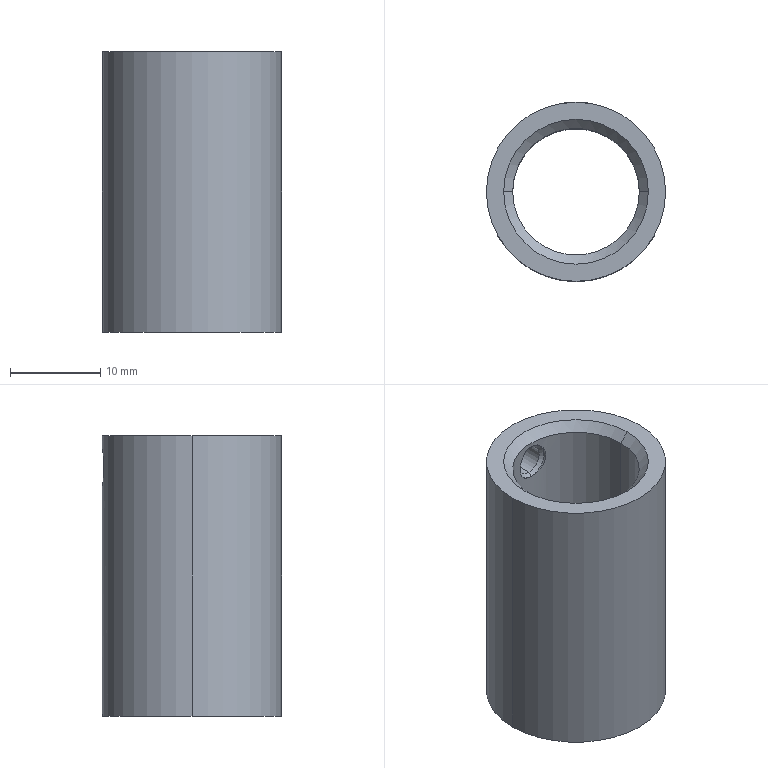Part | SolidWorks | features RefAxis 9, 3DProfileFeature 3, RevCut 1, Revolution 1 | 1 solid | 16 faces | box 19.8 x 19.8 x 31 mm | volume 4724 mm3 | cylinder 8 | cone 6 | plane 2 | commonest cylinder face diameters 3.242 x2 4 x2 14 x2 19.8 x2
STEP:
#1=CARTESIAN_POINT('',(0.,7.379,13.879));
#2=VERTEX_POINT('',#1);
#3=CARTESIAN_POINT('',(0.,7.379,17.121));
#4=VERTEX_POINT('',#3);
#5=CARTESIAN_POINT('',(0.,7.379,15.5));
#6=DIRECTION('',(0.,1.,0.));
#7=DIRECTION('',(0.,0.,1.));
#8=AXIS2_PLACEMENT_3D('',#5,#6,#7);
#9=CIRCLE('',#8,1.621);
#10=EDGE_CURVE('',#2,#4,#9,.T.);
#11=ORIENTED_EDGE('',*,*,#10,.T.);
#12=CARTESIAN_POINT('',(0.,7.,17.5));
#13=VERTEX_POINT('',#12);
#14=CARTESIAN_POINT('',(0.,7.,17.5));
#15=DIRECTION('',(0.,-0.7071,0.7071));
#16=VECTOR('',#15,1000.);
#17=LINE('',#14,#16);
#18=EDGE_CURVE('',#4,#13,#17,.T.);
#19=ORIENTED_EDGE('',*,*,#18,.T.);
#20=CARTESIAN_POINT('',(0.,7.,13.5));
#21=VERTEX_POINT('',#20);
#22=CARTESIAN_POINT('',(0.,7.,15.5));
#23=DIRECTION('',(0.,1.,0.));
#24=DIRECTION('',(0.,0.,1.));
#25=AXIS2_PLACEMENT_3D('',#22,#23,#24);
#26=CIRCLE('',#25,2.);
#27=EDGE_CURVE('',#21,#13,#26,.T.);
#28=ORIENTED_EDGE('',*,*,#27,.F.);
#29=CARTESIAN_POINT('',(0.,7.,13.5));
#30=DIRECTION('',(0.,-0.7071,-0.7071));
#31=VECTOR('',#30,1000.);
#32=LINE('',#29,#31);
#33=EDGE_CURVE('',#2,#21,#32,.T.);
#34=ORIENTED_EDGE('',*,*,#33,.F.);
#35=EDGE_LOOP('',(#11,#19,#28,#34));
#36=FACE_OUTER_BOUND('',#35,.T.);
#37=CARTESIAN_POINT('',(0.,7.,15.5));
#38=DIRECTION('',(0.,-1.,0.));
#39=DIRECTION('',(0.,0.,-1.));
#40=AXIS2_PLACEMENT_3D('',#37,#38,#39);
#41=CONICAL_SURFACE('',#40,2.,0.7854);
#42=ADVANCED_FACE('',(#36),#41,.F.);
#43=ORIENTED_EDGE('',*,*,#10,.F.);
#44=CARTESIAN_POINT('',(0.,9.521,13.879));
#45=VERTEX_POINT('',#44);
#46=CARTESIAN_POINT('',(0.,0.,13.879));
#47=DIRECTION('',(0.,1.,0.));
#48=VECTOR('',#47,1000.);
#49=LINE('',#46,#48);
#50=EDGE_CURVE('',#2,#45,#49,.T.);
#51=ORIENTED_EDGE('',*,*,#50,.T.);
#52=CARTESIAN_POINT('',(0.,9.521,17.121));
#53=VERTEX_POINT('',#52);
#54=CARTESIAN_POINT('',(0.,9.521,15.5));
#55=DIRECTION('',(0.,1.,0.));
#56=DIRECTION('',(0.,0.,1.));
#57=AXIS2_PLACEMENT_3D('',#54,#55,#56);
#58=CIRCLE('',#57,1.621);
#59=EDGE_CURVE('',#45,#53,#58,.T.);
#60=ORIENTED_EDGE('',*,*,#59,.T.);
#61=CARTESIAN_POINT('',(0.,0.,17.121));
#62=DIRECTION('',(0.,1.,0.));
#63=VECTOR('',#62,1000.);
#64=LINE('',#61,#63);
#65=EDGE_CURVE('',#4,#53,#64,.T.);
#66=ORIENTED_EDGE('',*,*,#65,.F.);
#67=EDGE_LOOP('',(#43,#51,#60,#66));
#68=FACE_OUTER_BOUND('',#67,.T.);
#69=CARTESIAN_POINT('',(0.,0.,15.5));
#70=DIRECTION('',(0.,1.,0.));
#71=DIRECTION('',(0.,0.,1.));
#72=AXIS2_PLACEMENT_3D('',#69,#70,#71);
#73=CYLINDRICAL_SURFACE('',#72,1.621);
#74=ADVANCED_FACE('',(#68),#73,.F.);
#75=ORIENTED_EDGE('',*,*,#59,.F.);
#76=CARTESIAN_POINT('',(0.,9.9,13.5));
#77=VERTEX_POINT('',#76);
#78=CARTESIAN_POINT('',(0.,9.521,13.879));
#79=DIRECTION('',(0.,0.7071,-0.7071));
#80=VECTOR('',#79,1000.);
#81=LINE('',#78,#80);
#82=EDGE_CURVE('',#45,#77,#81,.T.);
#83=ORIENTED_EDGE('',*,*,#82,.T.);
#84=CARTESIAN_POINT('',(0.,9.9,17.5));
#85=VERTEX_POINT('',#84);
#86=CARTESIAN_POINT('',(0.,9.9,13.5));
#87=CARTESIAN_POINT('',(-0.1265,9.9,13.5));
#88=CARTESIAN_POINT('',(-0.2509,9.898,13.514));
#89=CARTESIAN_POINT('',(-0.4957,9.888,13.57));
#90=CARTESIAN_POINT('',(-0.6163,9.881,13.613));
#91=CARTESIAN_POINT('',(-0.9551,9.856,13.774));
#92=CARTESIAN_POINT('',(-1.158,9.833,13.931));
#93=CARTESIAN_POINT('',(-1.407,9.8,14.217));
#94=CARTESIAN_POINT('',(-1.48,9.789,14.319));
#95=CARTESIAN_POINT('',(-1.606,9.769,14.535));
#96=CARTESIAN_POINT('',(-1.659,9.76,14.65));
#97=CARTESIAN_POINT('',(-1.744,9.745,14.886));
#98=CARTESIAN_POINT('',(-1.776,9.739,15.006));
#99=CARTESIAN_POINT('',(-1.819,9.731,15.254));
#100=CARTESIAN_POINT('',(-1.83,9.729,15.38));
#101=CARTESIAN_POINT('',(-1.829,9.73,15.631));
#102=CARTESIAN_POINT('',(-1.818,9.732,15.755));
#103=CARTESIAN_POINT('',(-1.774,9.74,16.002));
#104=CARTESIAN_POINT('',(-1.741,9.746,16.125));
#105=CARTESIAN_POINT('',(-1.655,9.761,16.359));
#106=CARTESIAN_POINT('',(-1.602,9.77,16.472));
#107=CARTESIAN_POINT('',(-1.475,9.79,16.688));
#108=CARTESIAN_POINT('',(-1.401,9.801,16.79));
#109=CARTESIAN_POINT('',(-1.155,9.834,17.07));
#110=CARTESIAN_POINT('',(-0.9517,9.857,17.228));
#111=CARTESIAN_POINT('',(-0.6148,9.882,17.388));
#112=CARTESIAN_POINT('',(-0.4953,9.888,17.43));
#113=CARTESIAN_POINT('',(-0.2495,9.898,17.486));
#114=CARTESIAN_POINT('',(-0.1254,9.9,17.5));
#115=CARTESIAN_POINT('',(0.,9.9,17.5));
#116=B_SPLINE_CURVE_WITH_KNOTS('',3,(#86,#87,#88,#89,#90,#91,#92,#93,#94,#95,#96,#97,#98,#99,#100,#101,#102,#103,#104,#105,#106,#107,#108,#109,#110,#111,#112,#113,#114,#115),.UNSPECIFIED.,.F.,.F.,(4,2,2,2,2,2,2,2,2,2,2,2,2,2,4),(0.01051,0.01088,0.01126,0.01201,0.01239,0.01276,0.01314,0.01352,0.01389,0.01427,0.01464,0.01502,0.01577,0.01615,0.01653),.UNSPECIFIED.);
#117=EDGE_CURVE('',#77,#85,#116,.T.);
#118=ORIENTED_EDGE('',*,*,#117,.T.);
#119=CARTESIAN_POINT('',(0.,9.521,17.121));
#120=DIRECTION('',(0.,0.7071,0.7071));
#121=VECTOR('',#120,1000.);
#122=LINE('',#119,#121);
#123=EDGE_CURVE('',#53,#85,#122,.T.);
#124=ORIENTED_EDGE('',*,*,#123,.F.);
#125=EDGE_LOOP('',(#75,#83,#118,#124));
#126=FACE_OUTER_BOUND('',#125,.T.);
#127=CARTESIAN_POINT('',(0.,9.521,15.5));
#128=DIRECTION('',(0.,1.,0.));
#129=DIRECTION('',(0.,0.,1.));
#130=AXIS2_PLACEMENT_3D('',#127,#128,#129);
#131=CONICAL_SURFACE('',#130,1.621,0.7854);
#132=ADVANCED_FACE('',(#126),#131,.F.);
#133=CARTESIAN_POINT('',(-7.,0.,18.));
#134=VERTEX_POINT('',#133);
#135=CARTESIAN_POINT('',(7.,0.,18.));
#136=VERTEX_POINT('',#135);
#137=CARTESIAN_POINT('',(0.,0.,18.));
#138=DIRECTION('',(0.,0.,1.));
#139=DIRECTION('',(1.,0.,0.));
#140=AXIS2_PLACEMENT_3D('',#137,#138,#139);
#141=CIRCLE('',#140,7.);
#142=EDGE_CURVE('',#134,#136,#141,.T.);
#143=ORIENTED_EDGE('',*,*,#142,.F.);
#144=CARTESIAN_POINT('',(-8.,0.,19.));
#145=VERTEX_POINT('',#144);
#146=CARTESIAN_POINT('',(-8.,0.,19.));
#147=DIRECTION('',(-0.7071,0.,0.7071));
#148=VECTOR('',#147,1000.);
#149=LINE('',#146,#148);
#150=EDGE_CURVE('',#134,#145,#149,.T.);
#151=ORIENTED_EDGE('',*,*,#150,.T.);
#152=CARTESIAN_POINT('',(8.,0.,19.));
#153=VERTEX_POINT('',#152);
#154=CARTESIAN_POINT('',(0.,0.,19.));
#155=DIRECTION('',(0.,0.,1.));
#156=DIRECTION('',(1.,0.,0.));
#157=AXIS2_PLACEMENT_3D('',#154,#155,#156);
#158=CIRCLE('',#157,8.);
#159=EDGE_CURVE('',#145,#153,#158,.T.);
#160=ORIENTED_EDGE('',*,*,#159,.T.);
#161=CARTESIAN_POINT('',(8.,0.,19.));
#162=DIRECTION('',(0.7071,0.,0.7071));
#163=VECTOR('',#162,1000.);
#164=LINE('',#161,#163);
#165=EDGE_CURVE('',#136,#153,#164,.T.);
#166=ORIENTED_EDGE('',*,*,#165,.F.);
#167=EDGE_LOOP('',(#143,#151,#160,#166));
#168=FACE_OUTER_BOUND('',#167,.T.);
#169=CARTESIAN_POINT('',(0.,0.,19.));
#170=DIRECTION('',(0.,0.,1.));
#171=DIRECTION('',(1.,0.,0.));
#172=AXIS2_PLACEMENT_3D('',#169,#170,#171);
#173=CONICAL_SURFACE('',#172,8.,0.7854);
#174=ADVANCED_FACE('',(#168),#173,.F.);
#175=CARTESIAN_POINT('',(0.,9.9,17.5));
#176=CARTESIAN_POINT('',(0.1254,9.9,17.5));
#177=CARTESIAN_POINT('',(0.2526,9.898,17.485));
#178=CARTESIAN_POINT('',(0.4965,9.888,17.429));
#179=CARTESIAN_POINT('',(0.6157,9.881,17.388));
#180=CARTESIAN_POINT('',(0.8433,9.865,17.279));
#181=CARTESIAN_POINT('',(0.9496,9.855,17.213));
#182=CARTESIAN_POINT('',(1.148,9.834,17.061));
#183=CARTESIAN_POINT('',(1.241,9.822,16.974));
#184=CARTESIAN_POINT('',(1.487,9.789,16.692));
#185=CARTESIAN_POINT('',(1.615,9.768,16.47));
#186=CARTESIAN_POINT('',(1.743,9.745,16.118));
#187=CARTESIAN_POINT('',(1.776,9.739,15.995));
#188=CARTESIAN_POINT('',(1.819,9.731,15.747));
#189=CARTESIAN_POINT('',(1.83,9.729,15.623));
#190=CARTESIAN_POINT('',(1.829,9.73,15.373));
#191=CARTESIAN_POINT('',(1.818,9.732,15.246));
#192=CARTESIAN_POINT('',(1.774,9.74,14.999));
#193=CARTESIAN_POINT('',(1.742,9.746,14.878));
#194=CARTESIAN_POINT('',(1.656,9.761,14.643));
#195=CARTESIAN_POINT('',(1.602,9.77,14.528));
#196=CARTESIAN_POINT('',(1.476,9.79,14.313));
#197=CARTESIAN_POINT('',(1.403,9.8,14.212));
#198=CARTESIAN_POINT('',(1.239,9.823,14.024));
#199=CARTESIAN_POINT('',(1.146,9.834,13.937));
#200=CARTESIAN_POINT('',(0.948,9.855,13.786));
#201=CARTESIAN_POINT('',(0.8421,9.865,13.72));
#202=CARTESIAN_POINT('',(0.6154,9.882,13.612));
#203=CARTESIAN_POINT('',(0.4953,9.888,13.57));
#204=CARTESIAN_POINT('',(0.2521,9.898,13.515));
#205=CARTESIAN_POINT('',(0.1265,9.9,13.5));
#206=CARTESIAN_POINT('',(0.,9.9,13.5));
#207=B_SPLINE_CURVE_WITH_KNOTS('',3,(#175,#176,#177,#178,#179,#180,#181,#182,#183,#184,#185,#186,#187,#188,#189,#190,#191,#192,#193,#194,#195,#196,#197,#198,#199,#200,#201,#202,#203,#204,#205,#206),.UNSPECIFIED.,.F.,.F.,(4,2,2,2,2,2,2,2,2,2,2,2,2,2,2,4),(0.004488,0.004864,0.00524,0.005616,0.005992,0.006745,0.007121,0.007497,0.007873,0.008249,0.008625,0.009002,0.009378,0.009754,0.01013,0.01051),.UNSPECIFIED.);
#208=EDGE_CURVE('',#85,#77,#207,.T.);
#209=ORIENTED_EDGE('',*,*,#208,.F.);
#210=ORIENTED_EDGE('',*,*,#117,.F.);
#211=EDGE_LOOP('',(#209,#210));
#212=FACE_BOUND('',#211,.T.);
#213=CARTESIAN_POINT('',(9.9,0.,-12.));
#214=VERTEX_POINT('',#213);
#215=CARTESIAN_POINT('',(-9.9,0.,-12.));
#216=VERTEX_POINT('',#215);
#217=CARTESIAN_POINT('',(0.,0.,-12.));
#218=DIRECTION('',(0.,0.,1.));
#219=DIRECTION('',(1.,0.,0.));
#220=AXIS2_PLACEMENT_3D('',#217,#218,#219);
#221=CIRCLE('',#220,9.9);
#222=EDGE_CURVE('',#214,#216,#221,.T.);
#223=ORIENTED_EDGE('',*,*,#222,.T.);
#224=CARTESIAN_POINT('',(-9.9,0.,19.));
#225=VERTEX_POINT('',#224);
#226=CARTESIAN_POINT('',(-9.9,0.,-12.));
#227=DIRECTION('',(0.,0.,1.));
#228=VECTOR('',#227,1000.);
#229=LINE('',#226,#228);
#230=EDGE_CURVE('',#216,#225,#229,.T.);
#231=ORIENTED_EDGE('',*,*,#230,.T.);
#232=CARTESIAN_POINT('',(9.9,0.,19.));
#233=VERTEX_POINT('',#232);
#234=CARTESIAN_POINT('',(0.,0.,19.));
#235=DIRECTION('',(0.,0.,1.));
#236=DIRECTION('',(1.,0.,0.));
#237=AXIS2_PLACEMENT_3D('',#234,#235,#236);
#238=CIRCLE('',#237,9.9);
#239=EDGE_CURVE('',#233,#225,#238,.T.);
#240=ORIENTED_EDGE('',*,*,#239,.F.);
#241=CARTESIAN_POINT('',(9.9,0.,-12.));
#242=DIRECTION('',(0.,0.,1.));
#243=VECTOR('',#242,1000.);
#244=LINE('',#241,#243);
#245=EDGE_CURVE('',#214,#233,#244,.T.);
#246=ORIENTED_EDGE('',*,*,#245,.F.);
#247=EDGE_LOOP('',(#223,#231,#240,#246));
#248=FACE_OUTER_BOUND('',#247,.T.);
#249=CARTESIAN_POINT('',(0.,0.,-12.));
#250=DIRECTION('',(0.,0.,1.));
#251=DIRECTION('',(1.,0.,0.));
#252=AXIS2_PLACEMENT_3D('',#249,#250,#251);
#253=CYLINDRICAL_SURFACE('',#252,9.9);
#254=ADVANCED_FACE('',(#212,#248),#253,.T.);
#255=CARTESIAN_POINT('',(-7.,0.,-12.));
#256=VERTEX_POINT('',#255);
#257=CARTESIAN_POINT('',(7.,0.,-12.));
#258=VERTEX_POINT('',#257);
#259=CARTESIAN_POINT('',(0.,0.,-12.));
#260=DIRECTION('',(0.,0.,1.));
#261=DIRECTION('',(1.,0.,0.));
#262=AXIS2_PLACEMENT_3D('',#259,#260,#261);
#263=CIRCLE('',#262,7.);
#264=EDGE_CURVE('',#256,#258,#263,.T.);
#265=ORIENTED_EDGE('',*,*,#264,.F.);
#266=CARTESIAN_POINT('',(-7.,0.,-12.));
#267=DIRECTION('',(0.,0.,1.));
#268=VECTOR('',#267,1000.);
#269=LINE('',#266,#268);
#270=EDGE_CURVE('',#256,#134,#269,.T.);
#271=ORIENTED_EDGE('',*,*,#270,.T.);
#272=ORIENTED_EDGE('',*,*,#142,.T.);
#273=CARTESIAN_POINT('',(7.,0.,-12.));
#274=DIRECTION('',(0.,0.,1.));
#275=VECTOR('',#274,1000.);
#276=LINE('',#273,#275);
#277=EDGE_CURVE('',#258,#136,#276,.T.);
#278=ORIENTED_EDGE('',*,*,#277,.F.);
#279=EDGE_LOOP('',(#265,#271,#272,#278));
#280=FACE_OUTER_BOUND('',#279,.T.);
#281=CARTESIAN_POINT('',(0.,0.,-12.));
#282=DIRECTION('',(0.,0.,1.));
#283=DIRECTION('',(1.,0.,0.));
#284=AXIS2_PLACEMENT_3D('',#281,#282,#283);
#285=CYLINDRICAL_SURFACE('',#284,7.);
#286=ADVANCED_FACE('',(#280),#285,.F.);
#287=ORIENTED_EDGE('',*,*,#270,.F.);
#288=CARTESIAN_POINT('',(0.,0.,-12.));
#289=DIRECTION('',(0.,0.,1.));
#290=DIRECTION('',(1.,0.,0.));
#291=AXIS2_PLACEMENT_3D('',#288,#289,#290);
#292=CIRCLE('',#291,7.);
#293=EDGE_CURVE('',#258,#256,#292,.T.);
#294=ORIENTED_EDGE('',*,*,#293,.F.);
#295=ORIENTED_EDGE('',*,*,#277,.T.);
#296=CARTESIAN_POINT('',(0.,0.,18.));
#297=DIRECTION('',(0.,0.,1.));
#298=DIRECTION('',(1.,0.,0.));
#299=AXIS2_PLACEMENT_3D('',#296,#297,#298);
#300=CIRCLE('',#299,7.);
#301=EDGE_CURVE('',#136,#134,#300,.T.);
#302=ORIENTED_EDGE('',*,*,#301,.T.);
#303=EDGE_LOOP('',(#287,#294,#295,#302));
#304=FACE_OUTER_BOUND('',#303,.T.);
#305=CARTESIAN_POINT('',(0.,7.,17.5));
#306=CARTESIAN_POINT('',(-0.1329,7.,17.5));
#307=CARTESIAN_POINT('',(-0.2634,6.996,17.487));
#308=CARTESIAN_POINT('',(-0.52,6.982,17.436));
#309=CARTESIAN_POINT('',(-0.6474,6.971,17.397));
#310=CARTESIAN_POINT('',(-0.8894,6.944,17.296));
#311=CARTESIAN_POINT('',(-1.004,6.928,17.235));
#312=CARTESIAN_POINT('',(-1.221,6.894,17.089));
#313=CARTESIAN_POINT('',(-1.323,6.874,17.005));
#314=CARTESIAN_POINT('',(-1.598,6.818,16.73));
#315=CARTESIAN_POINT('',(-1.747,6.779,16.508));
#316=CARTESIAN_POINT('',(-1.897,6.738,16.148));
#317=CARTESIAN_POINT('',(-1.935,6.727,16.021));
#318=CARTESIAN_POINT('',(-1.987,6.712,15.762));
#319=CARTESIAN_POINT('',(-2.,6.708,15.632));
#320=CARTESIAN_POINT('',(-2.,6.708,15.37));
#321=CARTESIAN_POINT('',(-1.987,6.712,15.236));
#322=CARTESIAN_POINT('',(-1.935,6.727,14.979));
#323=CARTESIAN_POINT('',(-1.897,6.738,14.854));
#324=CARTESIAN_POINT('',(-1.746,6.78,14.49));
#325=CARTESIAN_POINT('',(-1.599,6.818,14.27));
#326=CARTESIAN_POINT('',(-1.321,6.875,13.993));
#327=CARTESIAN_POINT('',(-1.221,6.894,13.911));
#328=CARTESIAN_POINT('',(-1.005,6.928,13.766));
#329=CARTESIAN_POINT('',(-0.8878,6.945,13.703));
#330=CARTESIAN_POINT('',(-0.6466,6.971,13.603));
#331=CARTESIAN_POINT('',(-0.5218,6.982,13.565));
#332=CARTESIAN_POINT('',(-0.2637,6.996,13.513));
#333=CARTESIAN_POINT('',(-0.131,7.,13.5));
#334=CARTESIAN_POINT('',(0.,7.,13.5));
#335=B_SPLINE_CURVE_WITH_KNOTS('',3,(#305,#306,#307,#308,#309,#310,#311,#312,#313,#314,#315,#316,#317,#318,#319,#320,#321,#322,#323,#324,#325,#326,#327,#328,#329,#330,#331,#332,#333,#334),.UNSPECIFIED.,.F.,.F.,(4,2,2,2,2,2,2,2,2,2,2,2,2,2,4),(0.,0.0003929,0.0007857,0.001179,0.001571,0.002357,0.00275,0.003143,0.003536,0.003929,0.004714,0.005107,0.0055,0.005893,0.006286),.UNSPECIFIED.);
#336=EDGE_CURVE('',#13,#21,#335,.T.);
#337=ORIENTED_EDGE('',*,*,#336,.F.);
#338=CARTESIAN_POINT('',(0.,7.,13.5));
#339=CARTESIAN_POINT('',(0.2619,7.,13.5));
#340=CARTESIAN_POINT('',(0.5263,6.984,13.553));
#341=CARTESIAN_POINT('',(0.8878,6.945,13.703));
#342=CARTESIAN_POINT('',(1.005,6.928,13.766));
#343=CARTESIAN_POINT('',(1.221,6.893,13.911));
#344=CARTESIAN_POINT('',(1.322,6.875,13.993));
#345=CARTESIAN_POINT('',(1.506,6.837,14.178));
#346=CARTESIAN_POINT('',(1.59,6.817,14.28));
#347=CARTESIAN_POINT('',(1.734,6.782,14.495));
#348=CARTESIAN_POINT('',(1.796,6.766,14.61));
#349=CARTESIAN_POINT('',(1.897,6.738,14.854));
#350=CARTESIAN_POINT('',(1.935,6.727,14.979));
#351=CARTESIAN_POINT('',(1.987,6.712,15.235));
#352=CARTESIAN_POINT('',(2.,6.708,15.368));
#353=CARTESIAN_POINT('',(2.,6.708,15.632));
#354=CARTESIAN_POINT('',(1.987,6.712,15.762));
#355=CARTESIAN_POINT('',(1.936,6.727,16.019));
#356=CARTESIAN_POINT('',(1.897,6.738,16.147));
#357=CARTESIAN_POINT('',(1.747,6.779,16.508));
#358=CARTESIAN_POINT('',(1.598,6.818,16.73));
#359=CARTESIAN_POINT('',(1.323,6.874,17.005));
#360=CARTESIAN_POINT('',(1.221,6.893,17.089));
#361=CARTESIAN_POINT('',(1.004,6.928,17.235));
#362=CARTESIAN_POINT('',(0.8897,6.944,17.296));
#363=CARTESIAN_POINT('',(0.6487,6.971,17.396));
#364=CARTESIAN_POINT('',(0.521,6.982,17.435));
#365=CARTESIAN_POINT('',(0.2636,6.996,17.487));
#366=CARTESIAN_POINT('',(0.1329,7.,17.5));
#367=CARTESIAN_POINT('',(0.,7.,17.5));
#368=B_SPLINE_CURVE_WITH_KNOTS('',3,(#338,#339,#340,#341,#342,#343,#344,#345,#346,#347,#348,#349,#350,#351,#352,#353,#354,#355,#356,#357,#358,#359,#360,#361,#362,#363,#364,#365,#366,#367),.UNSPECIFIED.,.F.,.F.,(4,2,2,2,2,2,2,2,2,2,2,2,2,2,4),(0.006286,0.007071,0.007464,0.007857,0.00825,0.008642,0.009035,0.009428,0.009821,0.01021,0.011,0.01139,0.01178,0.01218,0.01257),.UNSPECIFIED.);
#369=EDGE_CURVE('',#21,#13,#368,.T.);
#370=ORIENTED_EDGE('',*,*,#369,.F.);
#371=EDGE_LOOP('',(#337,#370));
#372=FACE_BOUND('',#371,.T.);
#373=CARTESIAN_POINT('',(0.,0.,-12.));
#374=DIRECTION('',(0.,0.,1.));
#375=DIRECTION('',(1.,0.,0.));
#376=AXIS2_PLACEMENT_3D('',#373,#374,#375);
#377=CYLINDRICAL_SURFACE('',#376,7.);
#378=ADVANCED_FACE('',(#304,#372),#377,.F.);
#379=ORIENTED_EDGE('',*,*,#230,.F.);
#380=CARTESIAN_POINT('',(0.,0.,-12.));
#381=DIRECTION('',(0.,0.,1.));
#382=DIRECTION('',(1.,0.,0.));
#383=AXIS2_PLACEMENT_3D('',#380,#381,#382);
#384=CIRCLE('',#383,9.9);
#385=EDGE_CURVE('',#216,#214,#384,.T.);
#386=ORIENTED_EDGE('',*,*,#385,.T.);
#387=ORIENTED_EDGE('',*,*,#245,.T.);
#388=CARTESIAN_POINT('',(0.,0.,19.));
#389=DIRECTION('',(0.,0.,1.));
#390=DIRECTION('',(1.,0.,0.));
#391=AXIS2_PLACEMENT_3D('',#388,#389,#390);
#392=CIRCLE('',#391,9.9);
#393=EDGE_CURVE('',#225,#233,#392,.T.);
#394=ORIENTED_EDGE('',*,*,#393,.F.);
#395=EDGE_LOOP('',(#379,#386,#387,#394));
#396=FACE_OUTER_BOUND('',#395,.T.);
#397=CARTESIAN_POINT('',(0.,0.,-12.));
#398=DIRECTION('',(0.,0.,1.));
#399=DIRECTION('',(1.,0.,0.));
#400=AXIS2_PLACEMENT_3D('',#397,#398,#399);
#401=CYLINDRICAL_SURFACE('',#400,9.9);
#402=ADVANCED_FACE('',(#396),#401,.T.);
#403=CARTESIAN_POINT('',(0.,0.,19.));
#404=DIRECTION('',(0.,0.,1.));
#405=DIRECTION('',(1.,0.,0.));
#406=AXIS2_PLACEMENT_3D('',#403,#404,#405);
#407=CIRCLE('',#406,8.);
#408=EDGE_CURVE('',#153,#145,#407,.T.);
#409=ORIENTED_EDGE('',*,*,#408,.F.);
#410=ORIENTED_EDGE('',*,*,#159,.F.);
#411=EDGE_LOOP('',(#409,#410));
#412=FACE_BOUND('',#411,.T.);
#413=ORIENTED_EDGE('',*,*,#239,.T.);
#414=ORIENTED_EDGE('',*,*,#393,.T.);
#415=EDGE_LOOP('',(#413,#414));
#416=FACE_OUTER_BOUND('',#415,.T.);
#417=CARTESIAN_POINT('',(0.,9.9,19.));
#418=DIRECTION('',(0.,0.,-1.));
#419=DIRECTION('',(-1.,0.,0.));
#420=AXIS2_PLACEMENT_3D('',#417,#418,#419);
#421=PLANE('',#420);
#422=ADVANCED_FACE('',(#412,#416),#421,.F.);
#423=ORIENTED_EDGE('',*,*,#150,.F.);
#424=ORIENTED_EDGE('',*,*,#301,.F.);
#425=ORIENTED_EDGE('',*,*,#165,.T.);
#426=ORIENTED_EDGE('',*,*,#408,.T.);
#427=EDGE_LOOP('',(#423,#424,#425,#426));
#428=FACE_OUTER_BOUND('',#427,.T.);
#429=CARTESIAN_POINT('',(0.,0.,19.));
#430=DIRECTION('',(0.,0.,1.));
#431=DIRECTION('',(1.,0.,0.));
#432=AXIS2_PLACEMENT_3D('',#429,#430,#431);
#433=CONICAL_SURFACE('',#432,8.,0.7854);
#434=ADVANCED_FACE('',(#428),#433,.F.);
#435=ORIENTED_EDGE('',*,*,#222,.F.);
#436=ORIENTED_EDGE('',*,*,#385,.F.);
#437=EDGE_LOOP('',(#435,#436));
#438=FACE_OUTER_BOUND('',#437,.T.);
#439=ORIENTED_EDGE('',*,*,#293,.T.);
#440=ORIENTED_EDGE('',*,*,#264,.T.);
#441=EDGE_LOOP('',(#439,#440));
#442=FACE_BOUND('',#441,.T.);
#443=CARTESIAN_POINT('',(0.,7.,-12.));
#444=DIRECTION('',(0.,0.,1.));
#445=DIRECTION('',(1.,0.,0.));
#446=AXIS2_PLACEMENT_3D('',#443,#444,#445);
#447=PLANE('',#446);
#448=ADVANCED_FACE('',(#438,#442),#447,.F.);
#449=ORIENTED_EDGE('',*,*,#336,.T.);
#450=ORIENTED_EDGE('',*,*,#27,.T.);
#451=EDGE_LOOP('',(#449,#450));
#452=FACE_OUTER_BOUND('',#451,.T.);
#453=CARTESIAN_POINT('',(0.,0.,15.5));
#454=DIRECTION('',(0.,1.,0.));
#455=DIRECTION('',(0.,0.,1.));
#456=AXIS2_PLACEMENT_3D('',#453,#454,#455);
#457=CYLINDRICAL_SURFACE('',#456,2.);
#458=ADVANCED_FACE('',(#452),#457,.F.);
#459=ORIENTED_EDGE('',*,*,#369,.T.);
#460=CARTESIAN_POINT('',(0.,7.,15.5));
#461=DIRECTION('',(0.,1.,0.));
#462=DIRECTION('',(0.,0.,1.));
#463=AXIS2_PLACEMENT_3D('',#460,#461,#462);
#464=CIRCLE('',#463,2.);
#465=EDGE_CURVE('',#13,#21,#464,.T.);
#466=ORIENTED_EDGE('',*,*,#465,.T.);
#467=EDGE_LOOP('',(#459,#466));
#468=FACE_OUTER_BOUND('',#467,.T.);
#469=CARTESIAN_POINT('',(0.,0.,15.5));
#470=DIRECTION('',(0.,1.,0.));
#471=DIRECTION('',(0.,0.,1.));
#472=AXIS2_PLACEMENT_3D('',#469,#470,#471);
#473=CYLINDRICAL_SURFACE('',#472,2.);
#474=ADVANCED_FACE('',(#468),#473,.F.);
#475=ORIENTED_EDGE('',*,*,#82,.F.);
#476=CARTESIAN_POINT('',(0.,9.521,15.5));
#477=DIRECTION('',(0.,1.,0.));
#478=DIRECTION('',(0.,0.,1.));
#479=AXIS2_PLACEMENT_3D('',#476,#477,#478);
#480=CIRCLE('',#479,1.621);
#481=EDGE_CURVE('',#53,#45,#480,.T.);
#482=ORIENTED_EDGE('',*,*,#481,.F.);
#483=ORIENTED_EDGE('',*,*,#123,.T.);
#484=ORIENTED_EDGE('',*,*,#208,.T.);
#485=EDGE_LOOP('',(#475,#482,#483,#484));
#486=FACE_OUTER_BOUND('',#485,.T.);
#487=CARTESIAN_POINT('',(0.,9.521,15.5));
#488=DIRECTION('',(0.,1.,0.));
#489=DIRECTION('',(0.,0.,1.));
#490=AXIS2_PLACEMENT_3D('',#487,#488,#489);
#491=CONICAL_SURFACE('',#490,1.621,0.7854);
#492=ADVANCED_FACE('',(#486),#491,.F.);
#493=ORIENTED_EDGE('',*,*,#50,.F.);
#494=CARTESIAN_POINT('',(0.,7.379,15.5));
#495=DIRECTION('',(0.,1.,0.));
#496=DIRECTION('',(0.,0.,1.));
#497=AXIS2_PLACEMENT_3D('',#494,#495,#496);
#498=CIRCLE('',#497,1.621);
#499=EDGE_CURVE('',#4,#2,#498,.T.);
#500=ORIENTED_EDGE('',*,*,#499,.F.);
#501=ORIENTED_EDGE('',*,*,#65,.T.);
#502=ORIENTED_EDGE('',*,*,#481,.T.);
#503=EDGE_LOOP('',(#493,#500,#501,#502));
#504=FACE_OUTER_BOUND('',#503,.T.);
#505=CARTESIAN_POINT('',(0.,0.,15.5));
#506=DIRECTION('',(0.,1.,0.));
#507=DIRECTION('',(0.,0.,1.));
#508=AXIS2_PLACEMENT_3D('',#505,#506,#507);
#509=CYLINDRICAL_SURFACE('',#508,1.621);
#510=ADVANCED_FACE('',(#504),#509,.F.);
#511=ORIENTED_EDGE('',*,*,#18,.F.);
#512=ORIENTED_EDGE('',*,*,#499,.T.);
#513=ORIENTED_EDGE('',*,*,#33,.T.);
#514=ORIENTED_EDGE('',*,*,#465,.F.);
#515=EDGE_LOOP('',(#511,#512,#513,#514));
#516=FACE_OUTER_BOUND('',#515,.T.);
#517=CARTESIAN_POINT('',(0.,7.,15.5));
#518=DIRECTION('',(0.,-1.,0.));
#519=DIRECTION('',(0.,0.,-1.));
#520=AXIS2_PLACEMENT_3D('',#517,#518,#519);
#521=CONICAL_SURFACE('',#520,2.,0.7854);
#522=ADVANCED_FACE('',(#516),#521,.F.);
#523=CLOSED_SHELL('',(#42,#74,#132,#174,#254,#286,#378,#402,#422,#434,#448,#458,#474,#492,#510,#522));
#524=MANIFOLD_SOLID_BREP('',#523);
#525=CARTESIAN_POINT('',(0.,0.,0.));
#526=DIRECTION('',(0.,0.,1.));
#527=DIRECTION('',(1.,0.,0.));
#528=AXIS2_PLACEMENT_3D('',#525,#526,#527);
#529=(LENGTH_UNIT()NAMED_UNIT(*)SI_UNIT(.MILLI.,.METRE.));
#530=UNCERTAINTY_MEASURE_WITH_UNIT(LENGTH_MEASURE(0.00001),#529,'','');
#531=(NAMED_UNIT(*)PLANE_ANGLE_UNIT()SI_UNIT($,.RADIAN.));
#532=(NAMED_UNIT(*)SI_UNIT($,.STERADIAN.)SOLID_ANGLE_UNIT());
#533=(GEOMETRIC_REPRESENTATION_CONTEXT(3)GLOBAL_UNCERTAINTY_ASSIGNED_CONTEXT((#530))GLOBAL_UNIT_ASSIGNED_CONTEXT((#529,#531,#532))REPRESENTATION_CONTEXT('',''));
#534=ADVANCED_BREP_SHAPE_REPRESENTATION('',(#524,#528),#533);